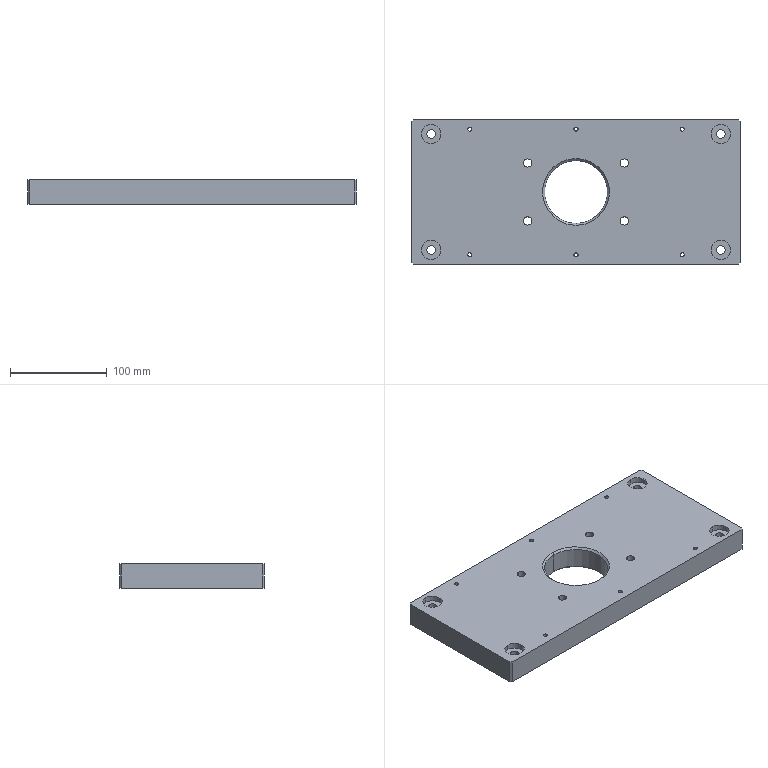NC program | NX | posted with a generic post | part box 340 x 150 x 25 mm
Whole program:
N10 G17 G21 G94 G90
(DRILLING_COPY_1 , TOOL : ZXZ)
N12 T01 M6
N14 G54
N16 G17 G0 G90 X-150. Y-60. S3000 M3
N18 G43 Z30. H1
N20 G94 G81 G98 Z-1. F200. R3.
N22 X-110. Y-65.
N24 X-50. Y-30.
N26 X0. Y-65.
N28 Y0.
N30 X50. Y-30.
N32 X110. Y-65.
N34 X150. Y-60.
N36 Y60.
N38 X110. Y65.
N40 X50. Y30.
N42 X0. Y65.
N44 X-50. Y30.
N46 X-110. Y65.
N48 X-150. Y60.
N50 G80
N52 G0 X-150. Y60. Z30.
N54 M5
(DRILLING_COPY_1_COPY_COPY_1_COPY_1 , TOOL : 9.0ZT)
N56 T09 M6
N58 G54
N60 G17 G0 G90 X-150. Y60. S1200 M3
N62 G43 Z30. H9
N64 G94 G83 G98 Z-29.204 F120. Q2. R3.
N66 Y-60.
N68 X0. Y0.
N70 X150. Y60.
N72 Y-60.
N74 G80
N76 G0 X150. Y-60. Z30.
N78 M5
(DRILLING_COPY_1_COPY_COPY_1_COPY_1_COPY , TOOL : 8.5ZT)
N80 T08 M6
N82 G54
N84 G17 G0 G90 X-50. Y-30. S1200 M3
N86 G43 Z30. H8
N88 G94 G83 G98 Z-29.054 F120. Q2. R3.
N90 Y30.
N92 X50.
N94 Y-30.
N96 G80
N98 G0 X50. Y-30. Z30.
N100 M5
(DRILLING_COPY_1_COPY_1 , TOOL : 4.2ZT)
N102 T14 M6
N104 G54
N106 G17 G0 G90 X-110. Y65. S2000 M3
N108 G43 Z30. H14
N110 G94 G83 G98 Z-24.262 F150. Q2. R3.
N112 X0.
N114 X110.
N116 Y-65.
N118 X0.
N120 X-110.
N122 G80
N124 G0 X-110. Y-65. Z30.
N126 M5
(HOLE_MILLING , TOOL : D16R0.8)
N128 T16 M6
N130 G54
N132 G17 G0 G90 X0. Y0. S2000 M3
N134 G43 Z30. H16
N136 Z0.5
N138 G94 G3 X4.083 Y-4.083 R4.083 F2000.
N140 X8.167 Y0. R4.083
N142 X8.167 Y0. Z0.25 I-8.167 J0.
N144 X8.167 Y0. Z0. I-8.167 J0.
N146 X8.167 Y0. Z-0.25 I-8.167 J0.
N148 X8.167 Y0. Z-0.5 I-8.167 J0.
N150 X8.167 Y0. Z-0.75 I-8.167 J0.
N152 X8.167 Y0. Z-1. I-8.167 J0.
N154 X8.167 Y0. Z-1.25 I-8.167 J0.
N156 X8.167 Y0. Z-1.5 I-8.167 J0.
N158 X8.167 Y0. Z-1.75 I-8.167 J0.
N160 X8.167 Y0. Z-2. I-8.167 J0.
N162 X8.167 Y0. Z-2.25 I-8.167 J0.
N164 X8.167 Y0. Z-2.5 I-8.167 J0.
N166 X8.167 Y0. Z-2.75 I-8.167 J0.
N168 X8.167 Y0. Z-3. I-8.167 J0.
N170 X8.167 Y0. Z-3.25 I-8.167 J0.
N172 X8.167 Y0. Z-3.5 I-8.167 J0.
N174 X8.167 Y0. Z-3.75 I-8.167 J0.
N176 X8.167 Y0. Z-4. I-8.167 J0.
N178 X8.167 Y0. Z-4.25 I-8.167 J0.
N180 X8.167 Y0. Z-4.5 I-8.167 J0.
N182 X8.167 Y0. Z-4.75 I-8.167 J0.
N184 X8.167 Y0. Z-5. I-8.167 J0.
N186 X8.167 Y0. Z-5.25 I-8.167 J0.
N188 X8.167 Y0. Z-5.5 I-8.167 J0.
N190 X8.167 Y0. Z-5.75 I-8.167 J0.
N192 X8.167 Y0. Z-6. I-8.167 J0.
N194 X8.167 Y0. Z-6.25 I-8.167 J0.
N196 X8.167 Y0. Z-6.5 I-8.167 J0.
N198 X8.167 Y0. Z-6.75 I-8.167 J0.
N200 X8.167 Y0. Z-7. I-8.167 J0.
N202 X8.167 Y0. Z-7.25 I-8.167 J0.
N204 X8.167 Y0. Z-7.5 I-8.167 J0.
N206 X8.167 Y0. Z-7.75 I-8.167 J0.
N208 X8.167 Y0. Z-8. I-8.167 J0.
N210 X8.167 Y0. Z-8.25 I-8.167 J0.
N212 X8.167 Y0. Z-8.5 I-8.167 J0.
N214 X8.167 Y0. Z-8.75 I-8.167 J0.
N216 X8.167 Y0. Z-9. I-8.167 J0.
N218 X8.167 Y0. Z-9.25 I-8.167 J0.
N220 X8.167 Y0. Z-9.5 I-8.167 J0.
N222 X8.167 Y0. Z-9.75 I-8.167 J0.
N224 X8.167 Y0. Z-10. I-8.167 J0.
N226 X8.167 Y0. Z-10.25 I-8.167 J0.
N228 X8.167 Y0. Z-10.5 I-8.167 J0.
N230 X8.167 Y0. Z-10.75 I-8.167 J0.
N232 X8.167 Y0. Z-11. I-8.167 J0.
N234 X8.167 Y0. Z-11.25 I-8.167 J0.
N236 X8.167 Y0. Z-11.5 I-8.167 J0.
N238 X8.167 Y0. Z-11.75 I-8.167 J0.
N240 X8.167 Y0. Z-12. I-8.167 J0.
N242 X8.167 Y0. Z-12.25 I-8.167 J0.
N244 X8.167 Y0. Z-12.5 I-8.167 J0.
N246 X8.167 Y0. Z-12.75 I-8.167 J0.
N248 X8.167 Y0. Z-13. I-8.167 J0.
N250 X8.167 Y0. Z-13.25 I-8.167 J0.
N252 X8.167 Y0. Z-13.5 I-8.167 J0.
N254 X8.167 Y0. Z-13.75 I-8.167 J0.
N256 X8.167 Y0. Z-14. I-8.167 J0.
N258 X8.167 Y0. Z-14.25 I-8.167 J0.
N260 X8.167 Y0. Z-14.5 I-8.167 J0.
N262 X8.167 Y0. Z-14.75 I-8.167 J0.
N264 X8.167 Y0. Z-15. I-8.167 J0.
N266 X8.167 Y0. Z-15.25 I-8.167 J0.
N268 X8.167 Y0. Z-15.5 I-8.167 J0.
N270 X8.167 Y0. Z-15.75 I-8.167 J0.
N272 X8.167 Y0. Z-16. I-8.167 J0.
N274 X8.167 Y0. Z-16.25 I-8.167 J0.
N276 X8.167 Y0. Z-16.5 I-8.167 J0.
N278 X8.167 Y0. Z-16.75 I-8.167 J0.
N280 X8.167 Y0. Z-17. I-8.167 J0.
N282 X8.167 Y0. Z-17.25 I-8.167 J0.
N284 X8.167 Y0. Z-17.5 I-8.167 J0.
N286 X8.167 Y0. Z-17.75 I-8.167 J0.
N288 X8.167 Y0. Z-18. I-8.167 J0.
N290 X8.167 Y0. Z-18.25 I-8.167 J0.
N292 X8.167 Y0. Z-18.5 I-8.167 J0.
N294 X8.167 Y0. Z-18.75 I-8.167 J0.
N296 X8.167 Y0. Z-19. I-8.167 J0.
N298 X8.167 Y0. Z-19.25 I-8.167 J0.
N300 X8.167 Y0. Z-19.5 I-8.167 J0.
N302 X8.167 Y0. Z-19.75 I-8.167 J0.
N304 X8.167 Y0. Z-20. I-8.167 J0.
N306 X8.167 Y0. Z-20.25 I-8.167 J0.
N308 X8.167 Y0. Z-20.5 I-8.167 J0.
N310 X8.167 Y0. Z-20.75 I-8.167 J0.
N312 X8.167 Y0. Z-21. I-8.167 J0.
N314 X8.167 Y0. Z-21.25 I-8.167 J0.
N316 X8.167 Y0. Z-21.5 I-8.167 J0.
N318 X8.167 Y0. Z-21.75 I-8.167 J0.
N320 X8.167 Y0. Z-22. I-8.167 J0.
N322 X8.167 Y0. Z-22.25 I-8.167 J0.
N324 X8.167 Y0. Z-22.5 I-8.167 J0.
N326 X8.167 Y0. Z-22.75 I-8.167 J0.
N328 X8.167 Y0. Z-23. I-8.167 J0.
N330 X8.167 Y0. Z-23.25 I-8.167 J0.
N332 X8.167 Y0. Z-23.5 I-8.167 J0.
N334 X8.167 Y0. Z-23.75 I-8.167 J0.
N336 X8.167 Y0. Z-24. I-8.167 J0.
N338 X8.167 Y0. Z-24.25 I-8.167 J0.
N340 X8.167 Y0. Z-24.5 I-8.167 J0.
N342 X8.167 Y0. Z-24.75 I-8.167 J0.
N344 X8.167 Y0. Z-25. I-8.167 J0.
N346 X8.167 Y0. Z-25.25 I-8.167 J0.
N348 X8.167 Y0. Z-25.5 I-8.167 J0.
N350 X8.167 Y0. Z-25.75 I-8.167 J0.
N352 X8.167 Y0. Z-26. I-8.167 J0.
N354 X0. Y8.167 R8.167
N356 X8.167 Y0. R-8.167
N358 X4.083 Y4.083 R4.083
N360 X0. Y0. R4.083
N362 G0 Z0.5
N364 G3 X8.167 Y-8.167 R8.167
N366 X16.333 Y0. R8.167
N368 X16.333 Y0. Z0.25 I-16.333 J0.
N370 X16.333 Y0. Z0. I-16.333 J0.
N372 X16.333 Y0. Z-0.25 I-16.333 J0.
N374 X16.333 Y0. Z-0.5 I-16.333 J0.
N376 X16.333 Y0. Z-0.75 I-16.333 J0.
N378 X16.333 Y0. Z-1. I-16.333 J0.
N380 X16.333 Y0. Z-1.25 I-16.333 J0.
N382 X16.333 Y0. Z-1.5 I-16.333 J0.
N384 X16.333 Y0. Z-1.75 I-16.333 J0.
N386 X16.333 Y0. Z-2. I-16.333 J0.
N388 X16.333 Y0. Z-2.25 I-16.333 J0.
N390 X16.333 Y0. Z-2.5 I-16.333 J0.
N392 X16.333 Y0. Z-2.75 I-16.333 J0.
N394 X16.333 Y0. Z-3. I-16.333 J0.
N396 X16.333 Y0. Z-3.25 I-16.333 J0.
N398 X16.333 Y0. Z-3.5 I-16.333 J0.
N400 X16.333 Y0. Z-3.75 I-16.333 J0.
N402 X16.333 Y0. Z-4. I-16.333 J0.
N404 X16.333 Y0. Z-4.25 I-16.333 J0.
N406 X16.333 Y0. Z-4.5 I-16.333 J0.
N408 X16.333 Y0. Z-4.75 I-16.333 J0.
N410 X16.333 Y0. Z-5. I-16.333 J0.
N412 X16.333 Y0. Z-5.25 I-16.333 J0.
N414 X16.333 Y0. Z-5.5 I-16.333 J0.
N416 X16.333 Y0. Z-5.75 I-16.333 J0.
N418 X16.333 Y0. Z-6. I-16.333 J0.
N420 X16.333 Y0. Z-6.25 I-16.333 J0.
N422 X16.333 Y0. Z-6.5 I-16.333 J0.
N424 X16.333 Y0. Z-6.75 I-16.333 J0.
N426 X16.333 Y0. Z-7. I-16.333 J0.
N428 X16.333 Y0. Z-7.25 I-16.333 J0.
N430 X16.333 Y0. Z-7.5 I-16.333 J0.
N432 X16.333 Y0. Z-7.75 I-16.333 J0.
N434 X16.333 Y0. Z-8. I-16.333 J0.
N436 X16.333 Y0. Z-8.25 I-16.333 J0.
N438 X16.333 Y0. Z-8.5 I-16.333 J0.
N440 X16.333 Y0. Z-8.75 I-16.333 J0.
N442 X16.333 Y0. Z-9. I-16.333 J0.
N444 X16.333 Y0. Z-9.25 I-16.333 J0.
N446 X16.333 Y0. Z-9.5 I-16.333 J0.
N448 X16.333 Y0. Z-9.75 I-16.333 J0.
N450 X16.333 Y0. Z-10. I-16.333 J0.
N452 X16.333 Y0. Z-10.25 I-16.333 J0.
N454 X16.333 Y0. Z-10.5 I-16.333 J0.
N456 X16.333 Y0. Z-10.75 I-16.333 J0.
N458 X16.333 Y0. Z-11. I-16.333 J0.
N460 X16.333 Y0. Z-11.25 I-16.333 J0.
N462 X16.333 Y0. Z-11.5 I-16.333 J0.
N464 X16.333 Y0. Z-11.75 I-16.333 J0.
N466 X16.333 Y0. Z-12. I-16.333 J0.
N468 X16.333 Y0. Z-12.25 I-16.333 J0.
N470 X16.333 Y0. Z-12.5 I-16.333 J0.
N472 X16.333 Y0. Z-12.75 I-16.333 J0.
N474 X16.333 Y0. Z-13. I-16.333 J0.
N476 X16.333 Y0. Z-13.25 I-16.333 J0.
N478 X16.333 Y0. Z-13.5 I-16.333 J0.
N480 X16.333 Y0. Z-13.75 I-16.333 J0.
N482 X16.333 Y0. Z-14. I-16.333 J0.
N484 X16.333 Y0. Z-14.25 I-16.333 J0.
N486 X16.333 Y0. Z-14.5 I-16.333 J0.
N488 X16.333 Y0. Z-14.75 I-16.333 J0.
N490 X16.333 Y0. Z-15. I-16.333 J0.
N492 X16.333 Y0. Z-15.25 I-16.333 J0.
N494 X16.333 Y0. Z-15.5 I-16.333 J0.
N496 X16.333 Y0. Z-15.75 I-16.333 J0.
N498 X16.333 Y0. Z-16. I-16.333 J0.
N500 X16.333 Y0. Z-16.25 I-16.333 J0.
N502 X16.333 Y0. Z-16.5 I-16.333 J0.
N504 X16.333 Y0. Z-16.75 I-16.333 J0.
N506 X16.333 Y0. Z-17. I-16.333 J0.
N508 X16.333 Y0. Z-17.25 I-16.333 J0.
N510 X16.333 Y0. Z-17.5 I-16.333 J0.
N512 X16.333 Y0. Z-17.75 I-16.333 J0.
N514 X16.333 Y0. Z-18. I-16.333 J0.
N516 X16.333 Y0. Z-18.25 I-16.333 J0.
N518 X16.333 Y0. Z-18.5 I-16.333 J0.
N520 X16.333 Y0. Z-18.75 I-16.333 J0.
N522 X16.333 Y0. Z-19. I-16.333 J0.
N524 X16.333 Y0. Z-19.25 I-16.333 J0.
N526 X16.333 Y0. Z-19.5 I-16.333 J0.
N528 X16.333 Y0. Z-19.75 I-16.333 J0.
N530 X16.333 Y0. Z-20. I-16.333 J0.
N532 X16.333 Y0. Z-20.25 I-16.333 J0.
N534 X16.333 Y0. Z-20.5 I-16.333 J0.
N536 X16.333 Y0. Z-20.75 I-16.333 J0.
N538 X16.333 Y0. Z-21. I-16.333 J0.
N540 X16.333 Y0. Z-21.25 I-16.333 J0.
N542 X16.333 Y0. Z-21.5 I-16.333 J0.
N544 X16.333 Y0. Z-21.75 I-16.333 J0.
N546 X16.333 Y0. Z-22. I-16.333 J0.
N548 X16.333 Y0. Z-22.25 I-16.333 J0.
N550 X16.333 Y0. Z-22.5 I-16.333 J0.
N552 X16.333 Y0. Z-22.75 I-16.333 J0.
N554 X16.333 Y0. Z-23. I-16.333 J0.
N556 X16.333 Y0. Z-23.25 I-16.333 J0.
N558 X16.333 Y0. Z-23.5 I-16.333 J0.
N560 X16.333 Y0. Z-23.75 I-16.333 J0.
N562 X16.333 Y0. Z-24. I-16.333 J0.
N564 X16.333 Y0. Z-24.25 I-16.333 J0.
N566 X16.333 Y0. Z-24.5 I-16.333 J0.
N568 X16.333 Y0. Z-24.75 I-16.333 J0.
N570 X16.333 Y0. Z-25. I-16.333 J0.
N572 X16.333 Y0. Z-25.25 I-16.333 J0.
N574 X16.333 Y0. Z-25.5 I-16.333 J0.
N576 X16.333 Y0. Z-25.75 I-16.333 J0.
N578 X16.333 Y0. Z-26. I-16.333 J0.
N580 X0. Y16.333 R16.333
N582 X16.333 Y0. R-16.333
N584 X8.167 Y8.167 R8.167
N586 X0. Y0. R8.167
N588 G0 Z0.5
N590 G3 X12.25 Y-12.25 R12.25
N592 X24.5 Y0. R12.25
N594 X24.5 Y0. Z0.25 I-24.5 J0.
N596 X24.5 Y0. Z0. I-24.5 J0.
N598 X24.5 Y0. Z-0.25 I-24.5 J0.
N600 X24.5 Y0. Z-0.5 I-24.5 J0.
N602 X24.5 Y0. Z-0.75 I-24.5 J0.
N604 X24.5 Y0. Z-1. I-24.5 J0.
N606 X24.5 Y0. Z-1.25 I-24.5 J0.
N608 X24.5 Y0. Z-1.5 I-24.5 J0.
N610 X24.5 Y0. Z-1.75 I-24.5 J0.
N612 X24.5 Y0. Z-2. I-24.5 J0.
N614 X24.5 Y0. Z-2.25 I-24.5 J0.
N616 X24.5 Y0. Z-2.5 I-24.5 J0.
N618 X24.5 Y0. Z-2.75 I-24.5 J0.
N620 X24.5 Y0. Z-3. I-24.5 J0.
N622 X24.5 Y0. Z-3.25 I-24.5 J0.
N624 X24.5 Y0. Z-3.5 I-24.5 J0.
N626 X24.5 Y0. Z-3.75 I-24.5 J0.
N628 X24.5 Y0. Z-4. I-24.5 J0.
N630 X24.5 Y0. Z-4.25 I-24.5 J0.
N632 X24.5 Y0. Z-4.5 I-24.5 J0.
N634 X24.5 Y0. Z-4.75 I-24.5 J0.
N636 X24.5 Y0. Z-5. I-24.5 J0.
N638 X24.5 Y0. Z-5.25 I-24.5 J0.
N640 X24.5 Y0. Z-5.5 I-24.5 J0.
N642 X24.5 Y0. Z-5.75 I-24.5 J0.
N644 X24.5 Y0. Z-6. I-24.5 J0.
N646 X24.5 Y0. Z-6.25 I-24.5 J0.
N648 X24.5 Y0. Z-6.5 I-24.5 J0.
N650 X24.5 Y0. Z-6.75 I-24.5 J0.
N652 X24.5 Y0. Z-7. I-24.5 J0.
N654 X24.5 Y0. Z-7.25 I-24.5 J0.
N656 X24.5 Y0. Z-7.5 I-24.5 J0.
N658 X24.5 Y0. Z-7.75 I-24.5 J0.
N660 X24.5 Y0. Z-8. I-24.5 J0.
N662 X24.5 Y0. Z-8.25 I-24.5 J0.
N664 X24.5 Y0. Z-8.5 I-24.5 J0.
N666 X24.5 Y0. Z-8.75 I-24.5 J0.
N668 X24.5 Y0. Z-9. I-24.5 J0.
N670 X24.5 Y0. Z-9.25 I-24.5 J0.
N672 X24.5 Y0. Z-9.5 I-24.5 J0.
N674 X24.5 Y0. Z-9.75 I-24.5 J0.
N676 X24.5 Y0. Z-10. I-24.5 J0.
N678 X24.5 Y0. Z-10.25 I-24.5 J0.
N680 X24.5 Y0. Z-10.5 I-24.5 J0.
N682 X24.5 Y0. Z-10.75 I-24.5 J0.
N684 X24.5 Y0. Z-11. I-24.5 J0.
N686 X24.5 Y0. Z-11.25 I-24.5 J0.
N688 X24.5 Y0. Z-11.5 I-24.5 J0.
N690 X24.5 Y0. Z-11.75 I-24.5 J0.
N692 X24.5 Y0. Z-12. I-24.5 J0.
N694 X24.5 Y0. Z-12.25 I-24.5 J0.
N696 X24.5 Y0. Z-12.5 I-24.5 J0.
N698 X24.5 Y0. Z-12.75 I-24.5 J0.
N700 X24.5 Y0. Z-13. I-24.5 J0.
N702 X24.5 Y0. Z-13.25 I-24.5 J0.
N704 X24.5 Y0. Z-13.5 I-24.5 J0.
N706 X24.5 Y0. Z-13.75 I-24.5 J0.
N708 X24.5 Y0. Z-14. I-24.5 J0.
N710 X24.5 Y0. Z-14.25 I-24.5 J0.
N712 X24.5 Y0. Z-14.5 I-24.5 J0.
N714 X24.5 Y0. Z-14.75 I-24.5 J0.
N716 X24.5 Y0. Z-15. I-24.5 J0.
N718 X24.5 Y0. Z-15.25 I-24.5 J0.
N720 X24.5 Y0. Z-15.5 I-24.5 J0.
N722 X24.5 Y0. Z-15.75 I-24.5 J0.
N724 X24.5 Y0. Z-16. I-24.5 J0.
N726 X24.5 Y0. Z-16.25 I-24.5 J0.
N728 X24.5 Y0. Z-16.5 I-24.5 J0.
N730 X24.5 Y0. Z-16.75 I-24.5 J0.
N732 X24.5 Y0. Z-17. I-24.5 J0.
N734 X24.5 Y0. Z-17.25 I-24.5 J0.
N736 X24.5 Y0. Z-17.5 I-24.5 J0.
N738 X24.5 Y0. Z-17.75 I-24.5 J0.
N740 X24.5 Y0. Z-18. I-24.5 J0.
N742 X24.5 Y0. Z-18.25 I-24.5 J0.
N744 X24.5 Y0. Z-18.5 I-24.5 J0.
N746 X24.5 Y0. Z-18.75 I-24.5 J0.
N748 X24.5 Y0. Z-19. I-24.5 J0.
N750 X24.5 Y0. Z-19.25 I-24.5 J0.
N752 X24.5 Y0. Z-19.5 I-24.5 J0.
N754 X24.5 Y0. Z-19.75 I-24.5 J0.
N756 X24.5 Y0. Z-20. I-24.5 J0.
N758 X24.5 Y0. Z-20.25 I-24.5 J0.
N760 X24.5 Y0. Z-20.5 I-24.5 J0.
N762 X24.5 Y0. Z-20.75 I-24.5 J0.
N764 X24.5 Y0. Z-21. I-24.5 J0.
N766 X24.5 Y0. Z-21.25 I-24.5 J0.
N768 X24.5 Y0. Z-21.5 I-24.5 J0.
N770 X24.5 Y0. Z-21.75 I-24.5 J0.
N772 X24.5 Y0. Z-22. I-24.5 J0.
N774 X24.5 Y0. Z-22.25 I-24.5 J0.
N776 X24.5 Y0. Z-22.5 I-24.5 J0.
N778 X24.5 Y0. Z-22.75 I-24.5 J0.
N780 X24.5 Y0. Z-23. I-24.5 J0.
N782 X24.5 Y0. Z-23.25 I-24.5 J0.
N784 X24.5 Y0. Z-23.5 I-24.5 J0.
N786 X24.5 Y0. Z-23.75 I-24.5 J0.
N788 X24.5 Y0. Z-24. I-24.5 J0.
N790 X24.5 Y0. Z-24.25 I-24.5 J0.
N792 X24.5 Y0. Z-24.5 I-24.5 J0.
N794 X24.5 Y0. Z-24.75 I-24.5 J0.
N796 X24.5 Y0. Z-25. I-24.5 J0.
N798 X24.5 Y0. Z-25.25 I-24.5 J0.
N800 X24.5 Y0. Z-25.5 I-24.5 J0.
N802 X24.5 Y0. Z-25.75 I-24.5 J0.
N804 X24.5 Y0. Z-26. I-24.5 J0.
N806 X0. Y24.5 R24.5
N808 X24.5 Y0. R-24.5
N810 X12.25 Y12.25 R12.25
N812 X0. Y0. R12.25
N814 G0 Z30.
(HOLE_MILLING_COPY , TOOL : D16R0.8)
N816 X-150. Y60.
N818 Z0.5
N820 G3 X-149.05 Y59.05 R0.95
N822 X-148.1 Y60. R0.95
N824 X-148.1 Y60. Z0.25 I-1.9 J0.
N826 X-148.1 Y60. Z0. I-1.9 J0.
N828 X-148.1 Y60. Z-0.25 I-1.9 J0.
N830 X-148.1 Y60. Z-0.5 I-1.9 J0.
N832 X-148.1 Y60. Z-0.75 I-1.9 J0.
N834 X-148.1 Y60. Z-1. I-1.9 J0.
N836 X-148.1 Y60. Z-1.25 I-1.9 J0.
N838 X-148.1 Y60. Z-1.5 I-1.9 J0.
N840 X-148.1 Y60. Z-1.75 I-1.9 J0.
N842 X-148.1 Y60. Z-2. I-1.9 J0.
N844 X-148.1 Y60. Z-2.25 I-1.9 J0.
N846 X-148.1 Y60. Z-2.5 I-1.9 J0.
N848 X-148.1 Y60. Z-2.75 I-1.9 J0.
N850 X-148.1 Y60. Z-3. I-1.9 J0.
N852 X-148.1 Y60. Z-3.25 I-1.9 J0.
N854 X-148.1 Y60. Z-3.5 I-1.9 J0.
N856 X-148.1 Y60. Z-3.75 I-1.9 J0.
N858 X-148.1 Y60. Z-4. I-1.9 J0.
N860 X-148.1 Y60. Z-4.25 I-1.9 J0.
N862 X-148.1 Y60. Z-4.5 I-1.9 J0.
N864 X-148.1 Y60. Z-4.75 I-1.9 J0.
N866 X-148.1 Y60. Z-5. I-1.9 J0.
N868 X-148.1 Y60. Z-5.25 I-1.9 J0.
N870 X-148.1 Y60. Z-5.5 I-1.9 J0.
N872 X-148.1 Y60. Z-5.75 I-1.9 J0.
N874 X-148.1 Y60. Z-6. I-1.9 J0.
N876 X-150. Y61.9 R1.9
N878 X-148.1 Y60. R-1.9
N880 X-149.05 Y60.95 R0.95
N882 X-150. Y60. R0.95
N884 G0 Z30.
N886 Y-60.
N888 Z0.5
N890 G3 X-149.05 Y-60.95 R0.95
N892 X-148.1 Y-60. R0.95
N894 X-148.1 Y-60. Z0.25 I-1.9 J0.
N896 X-148.1 Y-60. Z0. I-1.9 J0.
N898 X-148.1 Y-60. Z-0.25 I-1.9 J0.
N900 X-148.1 Y-60. Z-0.5 I-1.9 J0.
N902 X-148.1 Y-60. Z-0.75 I-1.9 J0.
N904 X-148.1 Y-60. Z-1. I-1.9 J0.
N906 X-148.1 Y-60. Z-1.25 I-1.9 J0.
N908 X-148.1 Y-60. Z-1.5 I-1.9 J0.
N910 X-148.1 Y-60. Z-1.75 I-1.9 J0.
N912 X-148.1 Y-60. Z-2. I-1.9 J0.
N914 X-148.1 Y-60. Z-2.25 I-1.9 J0.
N916 X-148.1 Y-60. Z-2.5 I-1.9 J0.
N918 X-148.1 Y-60. Z-2.75 I-1.9 J0.
N920 X-148.1 Y-60. Z-3. I-1.9 J0.
N922 X-148.1 Y-60. Z-3.25 I-1.9 J0.
N924 X-148.1 Y-60. Z-3.5 I-1.9 J0.
N926 X-148.1 Y-60. Z-3.75 I-1.9 J0.
N928 X-148.1 Y-60. Z-4. I-1.9 J0.
N930 X-148.1 Y-60. Z-4.25 I-1.9 J0.
N932 X-148.1 Y-60. Z-4.5 I-1.9 J0.
N934 X-148.1 Y-60. Z-4.75 I-1.9 J0.
N936 X-148.1 Y-60. Z-5. I-1.9 J0.
N938 X-148.1 Y-60. Z-5.25 I-1.9 J0.
N940 X-148.1 Y-60. Z-5.5 I-1.9 J0.
N942 X-148.1 Y-60. Z-5.75 I-1.9 J0.
N944 X-148.1 Y-60. Z-6. I-1.9 J0.
N946 X-150. Y-58.1 R1.9
N948 X-148.1 Y-60. R-1.9
N950 X-149.05 Y-59.05 R0.95
N952 X-150. Y-60. R0.95
N954 G0 Z30.
N956 X150. Y60.
N958 Z0.5
N960 G3 X150.95 Y59.05 R0.95
N962 X151.9 Y60. R0.95
N964 X151.9 Y60. Z0.25 I-1.9 J0.
N966 X151.9 Y60. Z0. I-1.9 J0.
N968 X151.9 Y60. Z-0.25 I-1.9 J0.
N970 X151.9 Y60. Z-0.5 I-1.9 J0.
N972 X151.9 Y60. Z-0.75 I-1.9 J0.
N974 X151.9 Y60. Z-1. I-1.9 J0.
N976 X151.9 Y60. Z-1.25 I-1.9 J0.
N978 X151.9 Y60. Z-1.5 I-1.9 J0.
N980 X151.9 Y60. Z-1.75 I-1.9 J0.
N982 X151.9 Y60. Z-2. I-1.9 J0.
N984 X151.9 Y60. Z-2.25 I-1.9 J0.
N986 X151.9 Y60. Z-2.5 I-1.9 J0.
N988 X151.9 Y60. Z-2.75 I-1.9 J0.
N990 X151.9 Y60. Z-3. I-1.9 J0.
N992 X151.9 Y60. Z-3.25 I-1.9 J0.
N994 X151.9 Y60. Z-3.5 I-1.9 J0.
N996 X151.9 Y60. Z-3.75 I-1.9 J0.
N998 X151.9 Y60. Z-4. I-1.9 J0.
N1000 X151.9 Y60. Z-4.25 I-1.9 J0.
N1002 X151.9 Y60. Z-4.5 I-1.9 J0.
N1004 X151.9 Y60. Z-4.75 I-1.9 J0.
N1006 X151.9 Y60. Z-5. I-1.9 J0.
N1008 X151.9 Y60. Z-5.25 I-1.9 J0.
N1010 X151.9 Y60. Z-5.5 I-1.9 J0.
N1012 X151.9 Y60. Z-5.75 I-1.9 J0.
N1014 X151.9 Y60. Z-6. I-1.9 J0.
N1016 X150. Y61.9 R1.9
N1018 X151.9 Y60. R-1.9
N1020 X150.95 Y60.95 R0.95
N1022 X150. Y60. R0.95
N1024 G0 Z30.
N1026 Y-60.
N1028 Z0.5
N1030 G3 X150.95 Y-60.95 R0.95
N1032 X151.9 Y-60. R0.95
N1034 X151.9 Y-60. Z0.25 I-1.9 J0.
N1036 X151.9 Y-60. Z0. I-1.9 J0.
N1038 X151.9 Y-60. Z-0.25 I-1.9 J0.
N1040 X151.9 Y-60. Z-0.5 I-1.9 J0.
N1042 X151.9 Y-60. Z-0.75 I-1.9 J0.
N1044 X151.9 Y-60. Z-1. I-1.9 J0.
N1046 X151.9 Y-60. Z-1.25 I-1.9 J0.
N1048 X151.9 Y-60. Z-1.5 I-1.9 J0.
N1050 X151.9 Y-60. Z-1.75 I-1.9 J0.
N1052 X151.9 Y-60. Z-2. I-1.9 J0.
N1054 X151.9 Y-60. Z-2.25 I-1.9 J0.
N1056 X151.9 Y-60. Z-2.5 I-1.9 J0.
N1058 X151.9 Y-60. Z-2.75 I-1.9 J0.
N1060 X151.9 Y-60. Z-3. I-1.9 J0.
N1062 X151.9 Y-60. Z-3.25 I-1.9 J0.
N1064 X151.9 Y-60. Z-3.5 I-1.9 J0.
N1066 X151.9 Y-60. Z-3.75 I-1.9 J0.
N1068 X151.9 Y-60. Z-4. I-1.9 J0.
N1070 X151.9 Y-60. Z-4.25 I-1.9 J0.
N1072 X151.9 Y-60. Z-4.5 I-1.9 J0.
N1074 X151.9 Y-60. Z-4.75 I-1.9 J0.
N1076 X151.9 Y-60. Z-5. I-1.9 J0.
N1078 X151.9 Y-60. Z-5.25 I-1.9 J0.
N1080 X151.9 Y-60. Z-5.5 I-1.9 J0.
N1082 X151.9 Y-60. Z-5.75 I-1.9 J0.
N1084 X151.9 Y-60. Z-6. I-1.9 J0.
N1086 X150. Y-58.1 R1.9
N1088 X151.9 Y-60. R-1.9
N1090 X150.95 Y-59.05 R0.95
N1092 X150. Y-60. R0.95
N1094 G0 Z30.
N1096 M5
(HOLE_MILLING_1 , TOOL : D10JING)
N1098 T11 M6
N1100 G54
N1102 G17 G0 G90 X24.327 Y-2.905 S5000 M3
N1104 G43 Z30. H11
N1106 Z-12.25
N1108 G94 G3 X27.6 Y0. R2.926 F850.
N1110 X0. Y27.6 R27.6
N1112 X27.6 Y0. R-27.6
N1114 X24.327 Y2.905 R2.926
N1116 G0 Y-2.905 Z-25.
N1118 G3 X27.6 Y0. R2.926
N1120 X0. Y27.6 R27.6
N1122 X27.6 Y0. R-27.6
N1124 X24.327 Y2.905 R2.926
N1126 G0 Z30.
N1128 M5
(ZLEVEL_PROFILE_COPY_1_COPY_COPY_COPY_COPY_2_COPY , TOOL : D6A45)
N1130 T07 M6
N1132 G54
N1134 G17 G0 G90 X-48.698 Y31.637 S4000 M3
N1136 G43 Z30. H7
N1138 Z-1.
N1140 G94 G1 X-49.48 Y32.991 F1000.
N1142 G3 X-50. Y33.291 R0.6
N1144 X-53.291 Y29.999 R3.291
N1146 X-50. Y33.291 R-3.291
N1148 X-50.52 Y32.991 R0.6
N1150 G1 X-51.302 Y31.637
N1152 G0 Z30.
N1154 X-110. Y66.141
N1156 Z0.
N1158 G1 Z-1.
N1160 G3 X-111.141 Y65. R1.141
N1162 X-110. Y66.141 R-1.141
N1164 X-110.52 Y65.841 R0.6
N1166 G0 Z30.
N1168 X0. Y66.141
N1170 Z0.
N1172 G1 Z-1.
N1174 X-0.003
N1176 G3 X-1.141 Y64.997 R1.141
N1178 X0. Y66.141 R-1.141
N1180 X-0.52 Y65.841 R0.6
N1182 G0 Z30.
N1184 X48.698 Y-31.637
N1186 Z-1.
N1188 G1 X49.48 Y-32.991
N1190 G3 X50. Y-33.291 R0.6
N1192 X53.291 Y-29.999 R3.291
N1194 X50. Y-33.291 R-3.291
N1196 X50.52 Y-32.991 R0.6
N1198 G1 X51.302 Y-31.637
N1200 G0 Z30.
N1202 X110. Y66.141
N1204 Z0.
N1206 G1 Z-1.
N1208 X109.995
N1210 G3 X108.859 Y64.995 R1.141
N1212 X110. Y66.141 R-1.141
N1214 X109.48 Y65.841 R0.6
N1216 G0 Z30.
N1218 X151.083 Y67.766
N1220 Z-1.
N1222 G1 X150.52 Y68.741
N1224 G3 X150. Y69.041 R0.6
N1226 X140.959 Y60. R9.041
N1228 X150. Y69.041 R-9.041
N1230 X149.48 Y68.741 R0.6
N1232 G1 X148.917 Y67.766
N1234 G0 Z30.
N1236 X-51.302 Y-31.637
N1238 Z-1.
N1240 G1 X-50.52 Y-32.991
N1242 G3 X-50. Y-33.291 R0.6
N1244 X-46.709 Y-30. R3.291
N1246 X-50. Y-33.291 R-3.291
N1248 X-49.48 Y-32.991 R0.6
N1250 G1 X-48.698 Y-31.637
N1252 G0 Z30.
N1254 X-148.917 Y67.766
N1256 Z-1.
N1258 G1 X-149.48 Y68.741
N1260 G3 X-150. Y69.041 R0.6
N1262 G1 X-150.001
N1264 G3 X-159.041 Y59.999 R9.041
N1266 X-150. Y69.041 R-9.041
N1268 X-150.52 Y68.741 R0.6
N1270 G1 X-151.083 Y67.766
N1272 G0 Z30.
N1274 X110. Y-66.141
N1276 Z0.
N1278 G1 Z-1.
N1280 G3 X111.141 Y-65. R1.141
N1282 X110. Y-66.141 R-1.141
N1284 X110.52 Y-65.841 R0.6
N1286 G0 Z30.
N1288 X0. Y-66.141
N1290 Z0.
N1292 G1 Z-1.
N1294 X0.003
N1296 G3 X1.141 Y-64.997 R1.141
N1298 X0. Y-66.141 R-1.141
N1300 X0.52 Y-65.841 R0.6
N1302 G0 Z30.
N1304 X-110. Y-66.141
N1306 Z0.
N1308 G1 Z-1.
N1310 X-109.995
N1312 G3 X-108.859 Y-64.995 R1.141
N1314 X-110. Y-66.141 R-1.141
N1316 X-109.48 Y-65.841 R0.6
N1318 G0 Z30.
N1320 X148.917 Y-67.766
N1322 Z-1.
N1324 G1 X149.48 Y-68.741
N1326 G3 X150. Y-69.041 R0.6
N1328 G1 X150.001
N1330 G3 X159.041 Y-59.999 R9.041
N1332 X150. Y-69.041 R-9.041
N1334 X150.52 Y-68.741 R0.6
N1336 G1 X151.083 Y-67.766
N1338 G0 Z30.
N1340 X-151.083
N1342 Z-1.
N1344 G1 X-150.52 Y-68.741
N1346 G3 X-150. Y-69.041 R0.6
N1348 X-140.959 Y-60. R9.041
N1350 X-150. Y-69.041 R-9.041
N1352 X-149.48 Y-68.741 R0.6
N1354 G1 X-148.917 Y-67.766
N1356 G0 Z30.
N1358 X51.302 Y31.637
N1360 Z-1.
N1362 G1 X50.52 Y32.991
N1364 G3 X50. Y33.291 R0.6
N1366 X46.709 Y30. R3.291
N1368 X50. Y33.291 R-3.291
N1370 X49.48 Y32.991 R0.6
N1372 G1 X48.698 Y31.637
N1374 G0 Z30.
(ZLEVEL_PROFILE_COPY_1_COPY_COPY_COPY_COPY_2_COPY_COPY , TOOL : D6A45)
N1376 X1.05 Y30.382
N1378 Z-2.5
N1380 G1 X0.52 Y31.3
N1382 G3 X0. Y31.6 R0.6
N1384 X-31.6 Y0. R31.6
N1386 X0. Y31.6 R-31.6
N1388 X-0.52 Y31.3 R0.6
N1390 G1 X-1.05 Y30.382
N1392 G0 Z30.
(ZLEVEL_PROFILE_COPY_1_COPY_COPY_COPY_COPY_2_COPY_COPY_COPY , TOOL : D6A45)
N1394 X1.05 Y30.882
N1396 Z-2.5
N1398 G1 X0.52 Y31.8
N1400 G3 X0. Y32.1 R0.6
N1402 G1 X-0.005
N1404 G3 X-32.1 Y-0.005 R32.1
N1406 X0. Y32.1 R-32.1
N1408 X-0.52 Y31.8 R0.6
N1410 G1 X-1.05 Y30.882
N1412 G0 Z30.
N1414 M5
(刀补11 , TOOL : D10JING)
N1416 T11 M6
N1418 G54
N1420 G17 G0 G90 X151.009 Y58.509 S5000 M3
N1422 G43 Z30. H11
N1424 Z-6.
N1426 G41 G94 G1 X151.065 Y58.427 F850. D11
N1428 G3 X154.95 Y60. R2.261
N1430 X150. Y64.95 R4.95
N1432 X154.95 Y60. R-4.95
N1434 X151.065 Y61.573 R2.261
N1436 G40
N1438 G1 X151.009 Y61.491
N1440 G0 Z30.
N1442 Y-61.491
N1444 Z-6.
N1446 G41 G1 X151.065 Y-61.573
N1448 G3 X154.95 Y-60. R2.261
N1450 X150. Y-55.05 R4.95
N1452 X154.95 Y-60. R-4.95
N1454 X151.065 Y-58.427 R2.261
N1456 G40
N1458 G1 X151.009 Y-58.509
N1460 G0 Z30.
N1462 X-148.991 Y58.509
N1464 Z-6.
N1466 G41 G1 X-148.935 Y58.427
N1468 G3 X-145.05 Y60. R2.261
N1470 X-150. Y64.95 R4.95
N1472 X-145.05 Y60. R-4.95
N1474 X-148.935 Y61.573 R2.261
N1476 G40
N1478 G1 X-148.991 Y61.491
N1480 G0 Z30.
N1482 Y-61.491
N1484 Z-6.
N1486 G41 G1 X-148.935 Y-61.573
N1488 G3 X-145.05 Y-60. R2.261
N1490 X-150. Y-55.05 R4.95
N1492 X-145.05 Y-60. R-4.95
N1494 X-148.935 Y-58.427 R2.261
N1496 G40
N1498 G1 X-148.991 Y-58.509
N1500 G0 Z30.
N1502 M5
N1504 M2